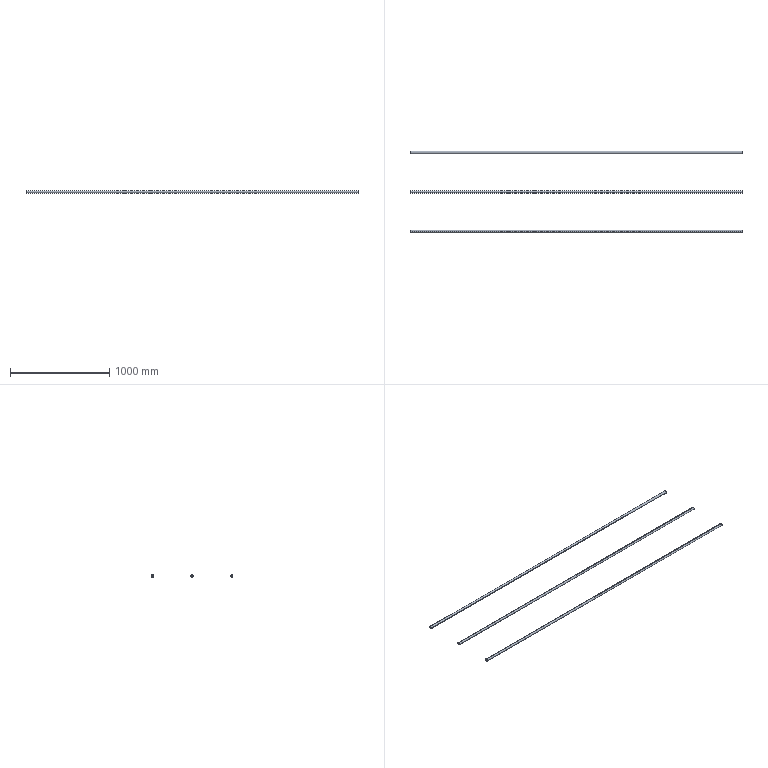Part | STEP file | 粉仓护栏栏杆7_Default<As Machined> | 3 solids | 18 faces | box 3350 x 825 x 25 mm | volume 1112948 mm3 | cylinder 12 | plane 6 | commonest cylinder face diameters 22 x6 25 x6
STEP:
#1=CARTESIAN_POINT('',(0.,0.,0.));
#2=DIRECTION('',(0.,0.,1.));
#3=DIRECTION('',(1.,0.,0.));
#4=AXIS2_PLACEMENT_3D('',#1,#2,#3);
#5=CARTESIAN_POINT('',(-3350.,0.,12.5));
#6=VERTEX_POINT('',#5);
#7=CARTESIAN_POINT('',(-3350.,0.,-12.5));
#8=VERTEX_POINT('',#7);
#9=CARTESIAN_POINT('',(-3350.,0.,0.));
#10=DIRECTION('',(-1.,0.,0.));
#11=DIRECTION('',(0.,-1.,0.));
#12=AXIS2_PLACEMENT_3D('',#9,#10,#11);
#13=CIRCLE('',#12,12.5);
#14=CARTESIAN_POINT('',(-3350.,0.,0.));
#15=DIRECTION('',(1.,0.,0.));
#16=DIRECTION('',(0.,0.,-1.));
#17=AXIS2_PLACEMENT_3D('',#14,#15,#16);
#18=CYLINDRICAL_SURFACE('',#17,12.5);
#19=CARTESIAN_POINT('',(4.712,0.));
#20=DIRECTION('',(-1.,0.));
#21=VECTOR('',#20,1.);
#22=LINE('',#19,#21);
#23=(GEOMETRIC_REPRESENTATION_CONTEXT(2)PARAMETRIC_REPRESENTATION_CONTEXT()REPRESENTATION_CONTEXT('',''));
#24=DEFINITIONAL_REPRESENTATION('',(#22),#23);
#25=PCURVE('',#18,#24);
#26=CARTESIAN_POINT('',(-3350.,0.,0.));
#27=DIRECTION('',(-1.,0.,0.));
#28=DIRECTION('',(0.,-1.,0.));
#29=AXIS2_PLACEMENT_3D('',#26,#27,#28);
#30=PLANE('',#29);
#31=CARTESIAN_POINT('',(0.,0.));
#32=DIRECTION('',(1.,0.));
#33=AXIS2_PLACEMENT_2D('',#31,#32);
#34=CIRCLE('',#33,12.5);
#35=(GEOMETRIC_REPRESENTATION_CONTEXT(2)PARAMETRIC_REPRESENTATION_CONTEXT()REPRESENTATION_CONTEXT('',''));
#36=DEFINITIONAL_REPRESENTATION('',(#34),#35);
#37=PCURVE('',#30,#36);
#38=SURFACE_CURVE('',#13,(#25,#37),.PCURVE_S1.);
#39=EDGE_CURVE('',#6,#8,#38,.T.);
#40=ORIENTED_EDGE('',*,*,#39,.F.);
#41=CARTESIAN_POINT('',(0.,0.,12.5));
#42=VERTEX_POINT('',#41);
#43=CARTESIAN_POINT('',(-3350.,0.,12.5));
#44=DIRECTION('',(1.,0.,0.));
#45=VECTOR('',#44,1.);
#46=LINE('',#43,#45);
#47=CARTESIAN_POINT('',(3.142,0.));
#48=DIRECTION('',(0.,1.));
#49=VECTOR('',#48,1.);
#50=LINE('',#47,#49);
#51=(GEOMETRIC_REPRESENTATION_CONTEXT(2)PARAMETRIC_REPRESENTATION_CONTEXT()REPRESENTATION_CONTEXT('',''));
#52=DEFINITIONAL_REPRESENTATION('',(#50),#51);
#53=PCURVE('',#18,#52);
#54=CARTESIAN_POINT('',(-3350.,0.,0.));
#55=DIRECTION('',(1.,0.,0.));
#56=DIRECTION('',(0.,0.,-1.));
#57=AXIS2_PLACEMENT_3D('',#54,#55,#56);
#58=CYLINDRICAL_SURFACE('',#57,12.5);
#59=CARTESIAN_POINT('',(3.142,0.));
#60=DIRECTION('',(0.,1.));
#61=VECTOR('',#60,1.);
#62=LINE('',#59,#61);
#63=(GEOMETRIC_REPRESENTATION_CONTEXT(2)PARAMETRIC_REPRESENTATION_CONTEXT()REPRESENTATION_CONTEXT('',''));
#64=DEFINITIONAL_REPRESENTATION('',(#62),#63);
#65=PCURVE('',#58,#64);
#66=SURFACE_CURVE('',#46,(#53,#65),.PCURVE_S1.);
#67=EDGE_CURVE('',#6,#42,#66,.T.);
#68=ORIENTED_EDGE('',*,*,#67,.T.);
#69=CARTESIAN_POINT('',(0.,0.,-12.5));
#70=VERTEX_POINT('',#69);
#71=CARTESIAN_POINT('',(0.,0.,0.));
#72=DIRECTION('',(-1.,0.,0.));
#73=DIRECTION('',(0.,-1.,0.));
#74=AXIS2_PLACEMENT_3D('',#71,#72,#73);
#75=CIRCLE('',#74,12.5);
#76=CARTESIAN_POINT('',(4.712,3350.));
#77=DIRECTION('',(-1.,0.));
#78=VECTOR('',#77,1.);
#79=LINE('',#76,#78);
#80=(GEOMETRIC_REPRESENTATION_CONTEXT(2)PARAMETRIC_REPRESENTATION_CONTEXT()REPRESENTATION_CONTEXT('',''));
#81=DEFINITIONAL_REPRESENTATION('',(#79),#80);
#82=PCURVE('',#18,#81);
#83=CARTESIAN_POINT('',(0.,0.,0.));
#84=DIRECTION('',(-1.,0.,0.));
#85=DIRECTION('',(0.,-1.,0.));
#86=AXIS2_PLACEMENT_3D('',#83,#84,#85);
#87=PLANE('',#86);
#88=CARTESIAN_POINT('',(0.,0.));
#89=DIRECTION('',(1.,0.));
#90=AXIS2_PLACEMENT_2D('',#88,#89);
#91=CIRCLE('',#90,12.5);
#92=(GEOMETRIC_REPRESENTATION_CONTEXT(2)PARAMETRIC_REPRESENTATION_CONTEXT()REPRESENTATION_CONTEXT('',''));
#93=DEFINITIONAL_REPRESENTATION('',(#91),#92);
#94=PCURVE('',#87,#93);
#95=SURFACE_CURVE('',#75,(#82,#94),.PCURVE_S1.);
#96=EDGE_CURVE('',#42,#70,#95,.T.);
#97=ORIENTED_EDGE('',*,*,#96,.T.);
#98=CARTESIAN_POINT('',(-3350.,0.,-12.5));
#99=DIRECTION('',(1.,0.,0.));
#100=VECTOR('',#99,1.);
#101=LINE('',#98,#100);
#102=CARTESIAN_POINT('',(0.,0.));
#103=DIRECTION('',(0.,1.));
#104=VECTOR('',#103,1.);
#105=LINE('',#102,#104);
#106=(GEOMETRIC_REPRESENTATION_CONTEXT(2)PARAMETRIC_REPRESENTATION_CONTEXT()REPRESENTATION_CONTEXT('',''));
#107=DEFINITIONAL_REPRESENTATION('',(#105),#106);
#108=PCURVE('',#18,#107);
#109=CARTESIAN_POINT('',(6.283,0.));
#110=DIRECTION('',(0.,1.));
#111=VECTOR('',#110,1.);
#112=LINE('',#109,#111);
#113=(GEOMETRIC_REPRESENTATION_CONTEXT(2)PARAMETRIC_REPRESENTATION_CONTEXT()REPRESENTATION_CONTEXT('',''));
#114=DEFINITIONAL_REPRESENTATION('',(#112),#113);
#115=PCURVE('',#58,#114);
#116=SURFACE_CURVE('',#101,(#108,#115),.PCURVE_S1.);
#117=EDGE_CURVE('',#8,#70,#116,.T.);
#118=ORIENTED_EDGE('',*,*,#117,.F.);
#119=EDGE_LOOP('',(#40,#68,#97,#118));
#120=FACE_BOUND('',#119,.T.);
#121=ADVANCED_FACE('',(#120),#18,.T.);
#122=CARTESIAN_POINT('',(-3350.,0.,-11.));
#123=VERTEX_POINT('',#122);
#124=CARTESIAN_POINT('',(0.,0.,-11.));
#125=VERTEX_POINT('',#124);
#126=CARTESIAN_POINT('',(-3350.,0.,-11.));
#127=DIRECTION('',(1.,0.,0.));
#128=VECTOR('',#127,1.);
#129=LINE('',#126,#128);
#130=CARTESIAN_POINT('',(-3350.,0.,0.));
#131=DIRECTION('',(1.,0.,0.));
#132=DIRECTION('',(0.,0.,-1.));
#133=AXIS2_PLACEMENT_3D('',#130,#131,#132);
#134=CYLINDRICAL_SURFACE('',#133,11.);
#135=CARTESIAN_POINT('',(6.283,0.));
#136=DIRECTION('',(0.,1.));
#137=VECTOR('',#136,1.);
#138=LINE('',#135,#137);
#139=(GEOMETRIC_REPRESENTATION_CONTEXT(2)PARAMETRIC_REPRESENTATION_CONTEXT()REPRESENTATION_CONTEXT('',''));
#140=DEFINITIONAL_REPRESENTATION('',(#138),#139);
#141=PCURVE('',#134,#140);
#142=CARTESIAN_POINT('',(-3350.,0.,0.));
#143=DIRECTION('',(1.,0.,0.));
#144=DIRECTION('',(0.,0.,-1.));
#145=AXIS2_PLACEMENT_3D('',#142,#143,#144);
#146=CYLINDRICAL_SURFACE('',#145,11.);
#147=CARTESIAN_POINT('',(0.,0.));
#148=DIRECTION('',(0.,1.));
#149=VECTOR('',#148,1.);
#150=LINE('',#147,#149);
#151=(GEOMETRIC_REPRESENTATION_CONTEXT(2)PARAMETRIC_REPRESENTATION_CONTEXT()REPRESENTATION_CONTEXT('',''));
#152=DEFINITIONAL_REPRESENTATION('',(#150),#151);
#153=PCURVE('',#146,#152);
#154=SURFACE_CURVE('',#129,(#141,#153),.PCURVE_S1.);
#155=EDGE_CURVE('',#123,#125,#154,.T.);
#156=ORIENTED_EDGE('',*,*,#155,.T.);
#157=CARTESIAN_POINT('',(0.,0.,11.));
#158=VERTEX_POINT('',#157);
#159=CARTESIAN_POINT('',(0.,0.,0.));
#160=DIRECTION('',(-1.,0.,0.));
#161=DIRECTION('',(0.,-1.,0.));
#162=AXIS2_PLACEMENT_3D('',#159,#160,#161);
#163=CIRCLE('',#162,11.);
#164=CARTESIAN_POINT('',(10.996,3350.));
#165=DIRECTION('',(-1.,0.));
#166=VECTOR('',#165,1.);
#167=LINE('',#164,#166);
#168=(GEOMETRIC_REPRESENTATION_CONTEXT(2)PARAMETRIC_REPRESENTATION_CONTEXT()REPRESENTATION_CONTEXT('',''));
#169=DEFINITIONAL_REPRESENTATION('',(#167),#168);
#170=PCURVE('',#134,#169);
#171=CARTESIAN_POINT('',(0.,0.));
#172=DIRECTION('',(1.,0.));
#173=AXIS2_PLACEMENT_2D('',#171,#172);
#174=CIRCLE('',#173,11.);
#175=(GEOMETRIC_REPRESENTATION_CONTEXT(2)PARAMETRIC_REPRESENTATION_CONTEXT()REPRESENTATION_CONTEXT('',''));
#176=DEFINITIONAL_REPRESENTATION('',(#174),#175);
#177=PCURVE('',#87,#176);
#178=SURFACE_CURVE('',#163,(#170,#177),.PCURVE_S1.);
#179=EDGE_CURVE('',#125,#158,#178,.T.);
#180=ORIENTED_EDGE('',*,*,#179,.T.);
#181=CARTESIAN_POINT('',(-3350.,0.,11.));
#182=VERTEX_POINT('',#181);
#183=CARTESIAN_POINT('',(-3350.,0.,11.));
#184=DIRECTION('',(1.,0.,0.));
#185=VECTOR('',#184,1.);
#186=LINE('',#183,#185);
#187=CARTESIAN_POINT('',(3.142,0.));
#188=DIRECTION('',(0.,1.));
#189=VECTOR('',#188,1.);
#190=LINE('',#187,#189);
#191=(GEOMETRIC_REPRESENTATION_CONTEXT(2)PARAMETRIC_REPRESENTATION_CONTEXT()REPRESENTATION_CONTEXT('',''));
#192=DEFINITIONAL_REPRESENTATION('',(#190),#191);
#193=PCURVE('',#134,#192);
#194=CARTESIAN_POINT('',(3.142,0.));
#195=DIRECTION('',(0.,1.));
#196=VECTOR('',#195,1.);
#197=LINE('',#194,#196);
#198=(GEOMETRIC_REPRESENTATION_CONTEXT(2)PARAMETRIC_REPRESENTATION_CONTEXT()REPRESENTATION_CONTEXT('',''));
#199=DEFINITIONAL_REPRESENTATION('',(#197),#198);
#200=PCURVE('',#146,#199);
#201=SURFACE_CURVE('',#186,(#193,#200),.PCURVE_S1.);
#202=EDGE_CURVE('',#182,#158,#201,.T.);
#203=ORIENTED_EDGE('',*,*,#202,.F.);
#204=CARTESIAN_POINT('',(-3350.,0.,0.));
#205=DIRECTION('',(-1.,0.,0.));
#206=DIRECTION('',(0.,-1.,0.));
#207=AXIS2_PLACEMENT_3D('',#204,#205,#206);
#208=CIRCLE('',#207,11.);
#209=CARTESIAN_POINT('',(10.996,0.));
#210=DIRECTION('',(-1.,0.));
#211=VECTOR('',#210,1.);
#212=LINE('',#209,#211);
#213=(GEOMETRIC_REPRESENTATION_CONTEXT(2)PARAMETRIC_REPRESENTATION_CONTEXT()REPRESENTATION_CONTEXT('',''));
#214=DEFINITIONAL_REPRESENTATION('',(#212),#213);
#215=PCURVE('',#134,#214);
#216=CARTESIAN_POINT('',(0.,0.));
#217=DIRECTION('',(1.,0.));
#218=AXIS2_PLACEMENT_2D('',#216,#217);
#219=CIRCLE('',#218,11.);
#220=(GEOMETRIC_REPRESENTATION_CONTEXT(2)PARAMETRIC_REPRESENTATION_CONTEXT()REPRESENTATION_CONTEXT('',''));
#221=DEFINITIONAL_REPRESENTATION('',(#219),#220);
#222=PCURVE('',#30,#221);
#223=SURFACE_CURVE('',#208,(#215,#222),.PCURVE_S1.);
#224=EDGE_CURVE('',#123,#182,#223,.T.);
#225=ORIENTED_EDGE('',*,*,#224,.F.);
#226=EDGE_LOOP('',(#156,#180,#203,#225));
#227=FACE_BOUND('',#226,.F.);
#228=ADVANCED_FACE('',(#227),#134,.F.);
#229=CARTESIAN_POINT('',(0.,0.,0.));
#230=DIRECTION('',(-1.,0.,0.));
#231=DIRECTION('',(0.,-1.,0.));
#232=AXIS2_PLACEMENT_3D('',#229,#230,#231);
#233=CIRCLE('',#232,11.);
#234=CARTESIAN_POINT('',(4.712,3350.));
#235=DIRECTION('',(-1.,0.));
#236=VECTOR('',#235,1.);
#237=LINE('',#234,#236);
#238=(GEOMETRIC_REPRESENTATION_CONTEXT(2)PARAMETRIC_REPRESENTATION_CONTEXT()REPRESENTATION_CONTEXT('',''));
#239=DEFINITIONAL_REPRESENTATION('',(#237),#238);
#240=PCURVE('',#146,#239);
#241=CARTESIAN_POINT('',(0.,0.));
#242=DIRECTION('',(1.,0.));
#243=AXIS2_PLACEMENT_2D('',#241,#242);
#244=CIRCLE('',#243,11.);
#245=(GEOMETRIC_REPRESENTATION_CONTEXT(2)PARAMETRIC_REPRESENTATION_CONTEXT()REPRESENTATION_CONTEXT('',''));
#246=DEFINITIONAL_REPRESENTATION('',(#244),#245);
#247=PCURVE('',#87,#246);
#248=SURFACE_CURVE('',#233,(#240,#247),.PCURVE_S1.);
#249=EDGE_CURVE('',#158,#125,#248,.T.);
#250=ORIENTED_EDGE('',*,*,#249,.T.);
#251=ORIENTED_EDGE('',*,*,#155,.F.);
#252=CARTESIAN_POINT('',(-3350.,0.,0.));
#253=DIRECTION('',(-1.,0.,0.));
#254=DIRECTION('',(0.,-1.,0.));
#255=AXIS2_PLACEMENT_3D('',#252,#253,#254);
#256=CIRCLE('',#255,11.);
#257=CARTESIAN_POINT('',(4.712,0.));
#258=DIRECTION('',(-1.,0.));
#259=VECTOR('',#258,1.);
#260=LINE('',#257,#259);
#261=(GEOMETRIC_REPRESENTATION_CONTEXT(2)PARAMETRIC_REPRESENTATION_CONTEXT()REPRESENTATION_CONTEXT('',''));
#262=DEFINITIONAL_REPRESENTATION('',(#260),#261);
#263=PCURVE('',#146,#262);
#264=CARTESIAN_POINT('',(0.,0.));
#265=DIRECTION('',(1.,0.));
#266=AXIS2_PLACEMENT_2D('',#264,#265);
#267=CIRCLE('',#266,11.);
#268=(GEOMETRIC_REPRESENTATION_CONTEXT(2)PARAMETRIC_REPRESENTATION_CONTEXT()REPRESENTATION_CONTEXT('',''));
#269=DEFINITIONAL_REPRESENTATION('',(#267),#268);
#270=PCURVE('',#30,#269);
#271=SURFACE_CURVE('',#256,(#263,#270),.PCURVE_S1.);
#272=EDGE_CURVE('',#182,#123,#271,.T.);
#273=ORIENTED_EDGE('',*,*,#272,.F.);
#274=ORIENTED_EDGE('',*,*,#202,.T.);
#275=EDGE_LOOP('',(#250,#251,#273,#274));
#276=FACE_BOUND('',#275,.F.);
#277=ADVANCED_FACE('',(#276),#146,.F.);
#278=ORIENTED_EDGE('',*,*,#67,.F.);
#279=CARTESIAN_POINT('',(-3350.,0.,0.));
#280=DIRECTION('',(-1.,0.,0.));
#281=DIRECTION('',(0.,-1.,0.));
#282=AXIS2_PLACEMENT_3D('',#279,#280,#281);
#283=CIRCLE('',#282,12.5);
#284=CARTESIAN_POINT('',(10.996,0.));
#285=DIRECTION('',(-1.,0.));
#286=VECTOR('',#285,1.);
#287=LINE('',#284,#286);
#288=(GEOMETRIC_REPRESENTATION_CONTEXT(2)PARAMETRIC_REPRESENTATION_CONTEXT()REPRESENTATION_CONTEXT('',''));
#289=DEFINITIONAL_REPRESENTATION('',(#287),#288);
#290=PCURVE('',#58,#289);
#291=CARTESIAN_POINT('',(0.,0.));
#292=DIRECTION('',(1.,0.));
#293=AXIS2_PLACEMENT_2D('',#291,#292);
#294=CIRCLE('',#293,12.5);
#295=(GEOMETRIC_REPRESENTATION_CONTEXT(2)PARAMETRIC_REPRESENTATION_CONTEXT()REPRESENTATION_CONTEXT('',''));
#296=DEFINITIONAL_REPRESENTATION('',(#294),#295);
#297=PCURVE('',#30,#296);
#298=SURFACE_CURVE('',#283,(#290,#297),.PCURVE_S1.);
#299=EDGE_CURVE('',#8,#6,#298,.T.);
#300=ORIENTED_EDGE('',*,*,#299,.F.);
#301=ORIENTED_EDGE('',*,*,#117,.T.);
#302=CARTESIAN_POINT('',(0.,0.,0.));
#303=DIRECTION('',(-1.,0.,0.));
#304=DIRECTION('',(0.,-1.,0.));
#305=AXIS2_PLACEMENT_3D('',#302,#303,#304);
#306=CIRCLE('',#305,12.5);
#307=CARTESIAN_POINT('',(10.996,3350.));
#308=DIRECTION('',(-1.,0.));
#309=VECTOR('',#308,1.);
#310=LINE('',#307,#309);
#311=(GEOMETRIC_REPRESENTATION_CONTEXT(2)PARAMETRIC_REPRESENTATION_CONTEXT()REPRESENTATION_CONTEXT('',''));
#312=DEFINITIONAL_REPRESENTATION('',(#310),#311);
#313=PCURVE('',#58,#312);
#314=CARTESIAN_POINT('',(0.,0.));
#315=DIRECTION('',(1.,0.));
#316=AXIS2_PLACEMENT_2D('',#314,#315);
#317=CIRCLE('',#316,12.5);
#318=(GEOMETRIC_REPRESENTATION_CONTEXT(2)PARAMETRIC_REPRESENTATION_CONTEXT()REPRESENTATION_CONTEXT('',''));
#319=DEFINITIONAL_REPRESENTATION('',(#317),#318);
#320=PCURVE('',#87,#319);
#321=SURFACE_CURVE('',#306,(#313,#320),.PCURVE_S1.);
#322=EDGE_CURVE('',#70,#42,#321,.T.);
#323=ORIENTED_EDGE('',*,*,#322,.T.);
#324=EDGE_LOOP('',(#278,#300,#301,#323));
#325=FACE_BOUND('',#324,.T.);
#326=ADVANCED_FACE('',(#325),#58,.T.);
#327=ORIENTED_EDGE('',*,*,#224,.F.);
#328=ORIENTED_EDGE('',*,*,#272,.F.);
#329=EDGE_LOOP('',(#327,#328));
#330=FACE_BOUND('',#329,.T.);
#331=ORIENTED_EDGE('',*,*,#299,.T.);
#332=ORIENTED_EDGE('',*,*,#39,.T.);
#333=EDGE_LOOP('',(#331,#332));
#334=FACE_BOUND('',#333,.T.);
#335=ADVANCED_FACE('',(#330,#334),#30,.T.);
#336=ORIENTED_EDGE('',*,*,#179,.T.);
#337=ORIENTED_EDGE('',*,*,#249,.T.);
#338=EDGE_LOOP('',(#336,#337));
#339=FACE_BOUND('',#338,.T.);
#340=ORIENTED_EDGE('',*,*,#322,.F.);
#341=ORIENTED_EDGE('',*,*,#96,.F.);
#342=EDGE_LOOP('',(#340,#341));
#343=FACE_BOUND('',#342,.T.);
#344=ADVANCED_FACE('',(#339,#343),#87,.F.);
#345=CLOSED_SHELL('',(#121,#228,#277,#326,#335,#344));
#346=MANIFOLD_SOLID_BREP('',#345);
#347=CARTESIAN_POINT('',(-3350.,787.5,0.));
#348=VERTEX_POINT('',#347);
#349=CARTESIAN_POINT('',(-3350.,812.5,0.));
#350=VERTEX_POINT('',#349);
#351=CARTESIAN_POINT('',(-3350.,800.,0.));
#352=DIRECTION('',(-1.,0.,0.));
#353=DIRECTION('',(0.,-1.,0.));
#354=AXIS2_PLACEMENT_3D('',#351,#352,#353);
#355=CIRCLE('',#354,12.5);
#356=CARTESIAN_POINT('',(-3350.,800.,0.));
#357=DIRECTION('',(1.,0.,0.));
#358=DIRECTION('',(0.,1.,0.));
#359=AXIS2_PLACEMENT_3D('',#356,#357,#358);
#360=CYLINDRICAL_SURFACE('',#359,12.5);
#361=CARTESIAN_POINT('',(3.142,0.));
#362=DIRECTION('',(-1.,0.));
#363=VECTOR('',#362,1.);
#364=LINE('',#361,#363);
#365=(GEOMETRIC_REPRESENTATION_CONTEXT(2)PARAMETRIC_REPRESENTATION_CONTEXT()REPRESENTATION_CONTEXT('',''));
#366=DEFINITIONAL_REPRESENTATION('',(#364),#365);
#367=PCURVE('',#360,#366);
#368=CARTESIAN_POINT('',(-3350.,800.,0.));
#369=DIRECTION('',(-1.,0.,0.));
#370=DIRECTION('',(0.,-1.,0.));
#371=AXIS2_PLACEMENT_3D('',#368,#369,#370);
#372=PLANE('',#371);
#373=CARTESIAN_POINT('',(0.,0.));
#374=DIRECTION('',(1.,0.));
#375=AXIS2_PLACEMENT_2D('',#373,#374);
#376=CIRCLE('',#375,12.5);
#377=(GEOMETRIC_REPRESENTATION_CONTEXT(2)PARAMETRIC_REPRESENTATION_CONTEXT()REPRESENTATION_CONTEXT('',''));
#378=DEFINITIONAL_REPRESENTATION('',(#376),#377);
#379=PCURVE('',#372,#378);
#380=SURFACE_CURVE('',#355,(#367,#379),.PCURVE_S1.);
#381=EDGE_CURVE('',#348,#350,#380,.T.);
#382=ORIENTED_EDGE('',*,*,#381,.F.);
#383=CARTESIAN_POINT('',(0.,787.5,0.));
#384=VERTEX_POINT('',#383);
#385=CARTESIAN_POINT('',(-3350.,787.5,0.));
#386=DIRECTION('',(1.,0.,0.));
#387=VECTOR('',#386,1.);
#388=LINE('',#385,#387);
#389=CARTESIAN_POINT('',(3.142,0.));
#390=DIRECTION('',(0.,1.));
#391=VECTOR('',#390,1.);
#392=LINE('',#389,#391);
#393=(GEOMETRIC_REPRESENTATION_CONTEXT(2)PARAMETRIC_REPRESENTATION_CONTEXT()REPRESENTATION_CONTEXT('',''));
#394=DEFINITIONAL_REPRESENTATION('',(#392),#393);
#395=PCURVE('',#360,#394);
#396=CARTESIAN_POINT('',(-3350.,800.,0.));
#397=DIRECTION('',(1.,0.,0.));
#398=DIRECTION('',(0.,1.,0.));
#399=AXIS2_PLACEMENT_3D('',#396,#397,#398);
#400=CYLINDRICAL_SURFACE('',#399,12.5);
#401=CARTESIAN_POINT('',(3.142,0.));
#402=DIRECTION('',(0.,1.));
#403=VECTOR('',#402,1.);
#404=LINE('',#401,#403);
#405=(GEOMETRIC_REPRESENTATION_CONTEXT(2)PARAMETRIC_REPRESENTATION_CONTEXT()REPRESENTATION_CONTEXT('',''));
#406=DEFINITIONAL_REPRESENTATION('',(#404),#405);
#407=PCURVE('',#400,#406);
#408=SURFACE_CURVE('',#388,(#395,#407),.PCURVE_S1.);
#409=EDGE_CURVE('',#348,#384,#408,.T.);
#410=ORIENTED_EDGE('',*,*,#409,.T.);
#411=CARTESIAN_POINT('',(0.,812.5,0.));
#412=VERTEX_POINT('',#411);
#413=CARTESIAN_POINT('',(0.,800.,0.));
#414=DIRECTION('',(-1.,0.,0.));
#415=DIRECTION('',(0.,-1.,0.));
#416=AXIS2_PLACEMENT_3D('',#413,#414,#415);
#417=CIRCLE('',#416,12.5);
#418=CARTESIAN_POINT('',(3.142,3350.));
#419=DIRECTION('',(-1.,0.));
#420=VECTOR('',#419,1.);
#421=LINE('',#418,#420);
#422=(GEOMETRIC_REPRESENTATION_CONTEXT(2)PARAMETRIC_REPRESENTATION_CONTEXT()REPRESENTATION_CONTEXT('',''));
#423=DEFINITIONAL_REPRESENTATION('',(#421),#422);
#424=PCURVE('',#360,#423);
#425=CARTESIAN_POINT('',(0.,800.,0.));
#426=DIRECTION('',(-1.,0.,0.));
#427=DIRECTION('',(0.,-1.,0.));
#428=AXIS2_PLACEMENT_3D('',#425,#426,#427);
#429=PLANE('',#428);
#430=CARTESIAN_POINT('',(0.,0.));
#431=DIRECTION('',(1.,0.));
#432=AXIS2_PLACEMENT_2D('',#430,#431);
#433=CIRCLE('',#432,12.5);
#434=(GEOMETRIC_REPRESENTATION_CONTEXT(2)PARAMETRIC_REPRESENTATION_CONTEXT()REPRESENTATION_CONTEXT('',''));
#435=DEFINITIONAL_REPRESENTATION('',(#433),#434);
#436=PCURVE('',#429,#435);
#437=SURFACE_CURVE('',#417,(#424,#436),.PCURVE_S1.);
#438=EDGE_CURVE('',#384,#412,#437,.T.);
#439=ORIENTED_EDGE('',*,*,#438,.T.);
#440=CARTESIAN_POINT('',(-3350.,812.5,0.));
#441=DIRECTION('',(1.,0.,0.));
#442=VECTOR('',#441,1.);
#443=LINE('',#440,#442);
#444=CARTESIAN_POINT('',(0.,0.));
#445=DIRECTION('',(0.,1.));
#446=VECTOR('',#445,1.);
#447=LINE('',#444,#446);
#448=(GEOMETRIC_REPRESENTATION_CONTEXT(2)PARAMETRIC_REPRESENTATION_CONTEXT()REPRESENTATION_CONTEXT('',''));
#449=DEFINITIONAL_REPRESENTATION('',(#447),#448);
#450=PCURVE('',#360,#449);
#451=CARTESIAN_POINT('',(6.283,0.));
#452=DIRECTION('',(0.,1.));
#453=VECTOR('',#452,1.);
#454=LINE('',#451,#453);
#455=(GEOMETRIC_REPRESENTATION_CONTEXT(2)PARAMETRIC_REPRESENTATION_CONTEXT()REPRESENTATION_CONTEXT('',''));
#456=DEFINITIONAL_REPRESENTATION('',(#454),#455);
#457=PCURVE('',#400,#456);
#458=SURFACE_CURVE('',#443,(#450,#457),.PCURVE_S1.);
#459=EDGE_CURVE('',#350,#412,#458,.T.);
#460=ORIENTED_EDGE('',*,*,#459,.F.);
#461=EDGE_LOOP('',(#382,#410,#439,#460));
#462=FACE_BOUND('',#461,.T.);
#463=ADVANCED_FACE('',(#462),#360,.T.);
#464=CARTESIAN_POINT('',(-3350.,811.,0.));
#465=VERTEX_POINT('',#464);
#466=CARTESIAN_POINT('',(0.,811.,0.));
#467=VERTEX_POINT('',#466);
#468=CARTESIAN_POINT('',(-3350.,811.,0.));
#469=DIRECTION('',(1.,0.,0.));
#470=VECTOR('',#469,1.);
#471=LINE('',#468,#470);
#472=CARTESIAN_POINT('',(-3350.,800.,0.));
#473=DIRECTION('',(1.,0.,0.));
#474=DIRECTION('',(0.,1.,0.));
#475=AXIS2_PLACEMENT_3D('',#472,#473,#474);
#476=CYLINDRICAL_SURFACE('',#475,11.);
#477=CARTESIAN_POINT('',(6.283,0.));
#478=DIRECTION('',(0.,1.));
#479=VECTOR('',#478,1.);
#480=LINE('',#477,#479);
#481=(GEOMETRIC_REPRESENTATION_CONTEXT(2)PARAMETRIC_REPRESENTATION_CONTEXT()REPRESENTATION_CONTEXT('',''));
#482=DEFINITIONAL_REPRESENTATION('',(#480),#481);
#483=PCURVE('',#476,#482);
#484=CARTESIAN_POINT('',(-3350.,800.,0.));
#485=DIRECTION('',(1.,0.,0.));
#486=DIRECTION('',(0.,1.,0.));
#487=AXIS2_PLACEMENT_3D('',#484,#485,#486);
#488=CYLINDRICAL_SURFACE('',#487,11.);
#489=CARTESIAN_POINT('',(0.,0.));
#490=DIRECTION('',(0.,1.));
#491=VECTOR('',#490,1.);
#492=LINE('',#489,#491);
#493=(GEOMETRIC_REPRESENTATION_CONTEXT(2)PARAMETRIC_REPRESENTATION_CONTEXT()REPRESENTATION_CONTEXT('',''));
#494=DEFINITIONAL_REPRESENTATION('',(#492),#493);
#495=PCURVE('',#488,#494);
#496=SURFACE_CURVE('',#471,(#483,#495),.PCURVE_S1.);
#497=EDGE_CURVE('',#465,#467,#496,.T.);
#498=ORIENTED_EDGE('',*,*,#497,.T.);
#499=CARTESIAN_POINT('',(0.,789.,0.));
#500=VERTEX_POINT('',#499);
#501=CARTESIAN_POINT('',(0.,800.,0.));
#502=DIRECTION('',(-1.,0.,0.));
#503=DIRECTION('',(0.,-1.,0.));
#504=AXIS2_PLACEMENT_3D('',#501,#502,#503);
#505=CIRCLE('',#504,11.);
#506=CARTESIAN_POINT('',(9.425,3350.));
#507=DIRECTION('',(-1.,0.));
#508=VECTOR('',#507,1.);
#509=LINE('',#506,#508);
#510=(GEOMETRIC_REPRESENTATION_CONTEXT(2)PARAMETRIC_REPRESENTATION_CONTEXT()REPRESENTATION_CONTEXT('',''));
#511=DEFINITIONAL_REPRESENTATION('',(#509),#510);
#512=PCURVE('',#476,#511);
#513=CARTESIAN_POINT('',(0.,0.));
#514=DIRECTION('',(1.,0.));
#515=AXIS2_PLACEMENT_2D('',#513,#514);
#516=CIRCLE('',#515,11.);
#517=(GEOMETRIC_REPRESENTATION_CONTEXT(2)PARAMETRIC_REPRESENTATION_CONTEXT()REPRESENTATION_CONTEXT('',''));
#518=DEFINITIONAL_REPRESENTATION('',(#516),#517);
#519=PCURVE('',#429,#518);
#520=SURFACE_CURVE('',#505,(#512,#519),.PCURVE_S1.);
#521=EDGE_CURVE('',#467,#500,#520,.T.);
#522=ORIENTED_EDGE('',*,*,#521,.T.);
#523=CARTESIAN_POINT('',(-3350.,789.,0.));
#524=VERTEX_POINT('',#523);
#525=CARTESIAN_POINT('',(-3350.,789.,0.));
#526=DIRECTION('',(1.,0.,0.));
#527=VECTOR('',#526,1.);
#528=LINE('',#525,#527);
#529=CARTESIAN_POINT('',(3.142,0.));
#530=DIRECTION('',(0.,1.));
#531=VECTOR('',#530,1.);
#532=LINE('',#529,#531);
#533=(GEOMETRIC_REPRESENTATION_CONTEXT(2)PARAMETRIC_REPRESENTATION_CONTEXT()REPRESENTATION_CONTEXT('',''));
#534=DEFINITIONAL_REPRESENTATION('',(#532),#533);
#535=PCURVE('',#476,#534);
#536=CARTESIAN_POINT('',(3.142,0.));
#537=DIRECTION('',(0.,1.));
#538=VECTOR('',#537,1.);
#539=LINE('',#536,#538);
#540=(GEOMETRIC_REPRESENTATION_CONTEXT(2)PARAMETRIC_REPRESENTATION_CONTEXT()REPRESENTATION_CONTEXT('',''));
#541=DEFINITIONAL_REPRESENTATION('',(#539),#540);
#542=PCURVE('',#488,#541);
#543=SURFACE_CURVE('',#528,(#535,#542),.PCURVE_S1.);
#544=EDGE_CURVE('',#524,#500,#543,.T.);
#545=ORIENTED_EDGE('',*,*,#544,.F.);
#546=CARTESIAN_POINT('',(-3350.,800.,0.));
#547=DIRECTION('',(-1.,0.,0.));
#548=DIRECTION('',(0.,-1.,0.));
#549=AXIS2_PLACEMENT_3D('',#546,#547,#548);
#550=CIRCLE('',#549,11.);
#551=CARTESIAN_POINT('',(9.425,0.));
#552=DIRECTION('',(-1.,0.));
#553=VECTOR('',#552,1.);
#554=LINE('',#551,#553);
#555=(GEOMETRIC_REPRESENTATION_CONTEXT(2)PARAMETRIC_REPRESENTATION_CONTEXT()REPRESENTATION_CONTEXT('',''));
#556=DEFINITIONAL_REPRESENTATION('',(#554),#555);
#557=PCURVE('',#476,#556);
#558=CARTESIAN_POINT('',(0.,0.));
#559=DIRECTION('',(1.,0.));
#560=AXIS2_PLACEMENT_2D('',#558,#559);
#561=CIRCLE('',#560,11.);
#562=(GEOMETRIC_REPRESENTATION_CONTEXT(2)PARAMETRIC_REPRESENTATION_CONTEXT()REPRESENTATION_CONTEXT('',''));
#563=DEFINITIONAL_REPRESENTATION('',(#561),#562);
#564=PCURVE('',#372,#563);
#565=SURFACE_CURVE('',#550,(#557,#564),.PCURVE_S1.);
#566=EDGE_CURVE('',#465,#524,#565,.T.);
#567=ORIENTED_EDGE('',*,*,#566,.F.);
#568=EDGE_LOOP('',(#498,#522,#545,#567));
#569=FACE_BOUND('',#568,.F.);
#570=ADVANCED_FACE('',(#569),#476,.F.);
#571=CARTESIAN_POINT('',(0.,800.,0.));
#572=DIRECTION('',(-1.,0.,0.));
#573=DIRECTION('',(0.,-1.,0.));
#574=AXIS2_PLACEMENT_3D('',#571,#572,#573);
#575=CIRCLE('',#574,11.);
#576=CARTESIAN_POINT('',(3.142,3350.));
#577=DIRECTION('',(-1.,0.));
#578=VECTOR('',#577,1.);
#579=LINE('',#576,#578);
#580=(GEOMETRIC_REPRESENTATION_CONTEXT(2)PARAMETRIC_REPRESENTATION_CONTEXT()REPRESENTATION_CONTEXT('',''));
#581=DEFINITIONAL_REPRESENTATION('',(#579),#580);
#582=PCURVE('',#488,#581);
#583=CARTESIAN_POINT('',(0.,0.));
#584=DIRECTION('',(1.,0.));
#585=AXIS2_PLACEMENT_2D('',#583,#584);
#586=CIRCLE('',#585,11.);
#587=(GEOMETRIC_REPRESENTATION_CONTEXT(2)PARAMETRIC_REPRESENTATION_CONTEXT()REPRESENTATION_CONTEXT('',''));
#588=DEFINITIONAL_REPRESENTATION('',(#586),#587);
#589=PCURVE('',#429,#588);
#590=SURFACE_CURVE('',#575,(#582,#589),.PCURVE_S1.);
#591=EDGE_CURVE('',#500,#467,#590,.T.);
#592=ORIENTED_EDGE('',*,*,#591,.T.);
#593=ORIENTED_EDGE('',*,*,#497,.F.);
#594=CARTESIAN_POINT('',(-3350.,800.,0.));
#595=DIRECTION('',(-1.,0.,0.));
#596=DIRECTION('',(0.,-1.,0.));
#597=AXIS2_PLACEMENT_3D('',#594,#595,#596);
#598=CIRCLE('',#597,11.);
#599=CARTESIAN_POINT('',(3.142,0.));
#600=DIRECTION('',(-1.,0.));
#601=VECTOR('',#600,1.);
#602=LINE('',#599,#601);
#603=(GEOMETRIC_REPRESENTATION_CONTEXT(2)PARAMETRIC_REPRESENTATION_CONTEXT()REPRESENTATION_CONTEXT('',''));
#604=DEFINITIONAL_REPRESENTATION('',(#602),#603);
#605=PCURVE('',#488,#604);
#606=CARTESIAN_POINT('',(0.,0.));
#607=DIRECTION('',(1.,0.));
#608=AXIS2_PLACEMENT_2D('',#606,#607);
#609=CIRCLE('',#608,11.);
#610=(GEOMETRIC_REPRESENTATION_CONTEXT(2)PARAMETRIC_REPRESENTATION_CONTEXT()REPRESENTATION_CONTEXT('',''));
#611=DEFINITIONAL_REPRESENTATION('',(#609),#610);
#612=PCURVE('',#372,#611);
#613=SURFACE_CURVE('',#598,(#605,#612),.PCURVE_S1.);
#614=EDGE_CURVE('',#524,#465,#613,.T.);
#615=ORIENTED_EDGE('',*,*,#614,.F.);
#616=ORIENTED_EDGE('',*,*,#544,.T.);
#617=EDGE_LOOP('',(#592,#593,#615,#616));
#618=FACE_BOUND('',#617,.F.);
#619=ADVANCED_FACE('',(#618),#488,.F.);
#620=ORIENTED_EDGE('',*,*,#409,.F.);
#621=CARTESIAN_POINT('',(-3350.,800.,0.));
#622=DIRECTION('',(-1.,0.,0.));
#623=DIRECTION('',(0.,-1.,0.));
#624=AXIS2_PLACEMENT_3D('',#621,#622,#623);
#625=CIRCLE('',#624,12.5);
#626=CARTESIAN_POINT('',(9.425,0.));
#627=DIRECTION('',(-1.,0.));
#628=VECTOR('',#627,1.);
#629=LINE('',#626,#628);
#630=(GEOMETRIC_REPRESENTATION_CONTEXT(2)PARAMETRIC_REPRESENTATION_CONTEXT()REPRESENTATION_CONTEXT('',''));
#631=DEFINITIONAL_REPRESENTATION('',(#629),#630);
#632=PCURVE('',#400,#631);
#633=CARTESIAN_POINT('',(0.,0.));
#634=DIRECTION('',(1.,0.));
#635=AXIS2_PLACEMENT_2D('',#633,#634);
#636=CIRCLE('',#635,12.5);
#637=(GEOMETRIC_REPRESENTATION_CONTEXT(2)PARAMETRIC_REPRESENTATION_CONTEXT()REPRESENTATION_CONTEXT('',''));
#638=DEFINITIONAL_REPRESENTATION('',(#636),#637);
#639=PCURVE('',#372,#638);
#640=SURFACE_CURVE('',#625,(#632,#639),.PCURVE_S1.);
#641=EDGE_CURVE('',#350,#348,#640,.T.);
#642=ORIENTED_EDGE('',*,*,#641,.F.);
#643=ORIENTED_EDGE('',*,*,#459,.T.);
#644=CARTESIAN_POINT('',(0.,800.,0.));
#645=DIRECTION('',(-1.,0.,0.));
#646=DIRECTION('',(0.,-1.,0.));
#647=AXIS2_PLACEMENT_3D('',#644,#645,#646);
#648=CIRCLE('',#647,12.5);
#649=CARTESIAN_POINT('',(9.425,3350.));
#650=DIRECTION('',(-1.,0.));
#651=VECTOR('',#650,1.);
#652=LINE('',#649,#651);
#653=(GEOMETRIC_REPRESENTATION_CONTEXT(2)PARAMETRIC_REPRESENTATION_CONTEXT()REPRESENTATION_CONTEXT('',''));
#654=DEFINITIONAL_REPRESENTATION('',(#652),#653);
#655=PCURVE('',#400,#654);
#656=CARTESIAN_POINT('',(0.,0.));
#657=DIRECTION('',(1.,0.));
#658=AXIS2_PLACEMENT_2D('',#656,#657);
#659=CIRCLE('',#658,12.5);
#660=(GEOMETRIC_REPRESENTATION_CONTEXT(2)PARAMETRIC_REPRESENTATION_CONTEXT()REPRESENTATION_CONTEXT('',''));
#661=DEFINITIONAL_REPRESENTATION('',(#659),#660);
#662=PCURVE('',#429,#661);
#663=SURFACE_CURVE('',#648,(#655,#662),.PCURVE_S1.);
#664=EDGE_CURVE('',#412,#384,#663,.T.);
#665=ORIENTED_EDGE('',*,*,#664,.T.);
#666=EDGE_LOOP('',(#620,#642,#643,#665));
#667=FACE_BOUND('',#666,.T.);
#668=ADVANCED_FACE('',(#667),#400,.T.);
#669=ORIENTED_EDGE('',*,*,#566,.F.);
#670=ORIENTED_EDGE('',*,*,#614,.F.);
#671=EDGE_LOOP('',(#669,#670));
#672=FACE_BOUND('',#671,.T.);
#673=ORIENTED_EDGE('',*,*,#641,.T.);
#674=ORIENTED_EDGE('',*,*,#381,.T.);
#675=EDGE_LOOP('',(#673,#674));
#676=FACE_BOUND('',#675,.T.);
#677=ADVANCED_FACE('',(#672,#676),#372,.T.);
#678=ORIENTED_EDGE('',*,*,#521,.T.);
#679=ORIENTED_EDGE('',*,*,#591,.T.);
#680=EDGE_LOOP('',(#678,#679));
#681=FACE_BOUND('',#680,.T.);
#682=ORIENTED_EDGE('',*,*,#664,.F.);
#683=ORIENTED_EDGE('',*,*,#438,.F.);
#684=EDGE_LOOP('',(#682,#683));
#685=FACE_BOUND('',#684,.T.);
#686=ADVANCED_FACE('',(#681,#685),#429,.F.);
#687=CLOSED_SHELL('',(#463,#570,#619,#668,#677,#686));
#688=MANIFOLD_SOLID_BREP('',#687);
#689=CARTESIAN_POINT('',(0.,400.,-12.5));
#690=VERTEX_POINT('',#689);
#691=CARTESIAN_POINT('',(0.,400.,12.5));
#692=VERTEX_POINT('',#691);
#693=CARTESIAN_POINT('',(0.,400.,0.));
#694=DIRECTION('',(1.,0.,0.));
#695=DIRECTION('',(0.,1.,0.));
#696=AXIS2_PLACEMENT_3D('',#693,#694,#695);
#697=CIRCLE('',#696,12.5);
#698=CARTESIAN_POINT('',(0.,400.,0.));
#699=DIRECTION('',(-1.,0.,0.));
#700=DIRECTION('',(0.,0.,1.));
#701=AXIS2_PLACEMENT_3D('',#698,#699,#700);
#702=CYLINDRICAL_SURFACE('',#701,12.5);
#703=CARTESIAN_POINT('',(7.854,0.));
#704=DIRECTION('',(-1.,0.));
#705=VECTOR('',#704,1.);
#706=LINE('',#703,#705);
#707=(GEOMETRIC_REPRESENTATION_CONTEXT(2)PARAMETRIC_REPRESENTATION_CONTEXT()REPRESENTATION_CONTEXT('',''));
#708=DEFINITIONAL_REPRESENTATION('',(#706),#707);
#709=PCURVE('',#702,#708);
#710=CARTESIAN_POINT('',(0.,400.,0.));
#711=DIRECTION('',(1.,0.,0.));
#712=DIRECTION('',(0.,1.,0.));
#713=AXIS2_PLACEMENT_3D('',#710,#711,#712);
#714=PLANE('',#713);
#715=CARTESIAN_POINT('',(0.,0.));
#716=DIRECTION('',(1.,0.));
#717=AXIS2_PLACEMENT_2D('',#715,#716);
#718=CIRCLE('',#717,12.5);
#719=(GEOMETRIC_REPRESENTATION_CONTEXT(2)PARAMETRIC_REPRESENTATION_CONTEXT()REPRESENTATION_CONTEXT('',''));
#720=DEFINITIONAL_REPRESENTATION('',(#718),#719);
#721=PCURVE('',#714,#720);
#722=SURFACE_CURVE('',#697,(#709,#721),.PCURVE_S1.);
#723=EDGE_CURVE('',#690,#692,#722,.T.);
#724=ORIENTED_EDGE('',*,*,#723,.F.);
#725=CARTESIAN_POINT('',(-3350.,400.,-12.5));
#726=VERTEX_POINT('',#725);
#727=CARTESIAN_POINT('',(0.,400.,-12.5));
#728=DIRECTION('',(-1.,0.,0.));
#729=VECTOR('',#728,1.);
#730=LINE('',#727,#729);
#731=CARTESIAN_POINT('',(3.142,0.));
#732=DIRECTION('',(0.,1.));
#733=VECTOR('',#732,1.);
#734=LINE('',#731,#733);
#735=(GEOMETRIC_REPRESENTATION_CONTEXT(2)PARAMETRIC_REPRESENTATION_CONTEXT()REPRESENTATION_CONTEXT('',''));
#736=DEFINITIONAL_REPRESENTATION('',(#734),#735);
#737=PCURVE('',#702,#736);
#738=CARTESIAN_POINT('',(0.,400.,0.));
#739=DIRECTION('',(-1.,0.,0.));
#740=DIRECTION('',(0.,0.,1.));
#741=AXIS2_PLACEMENT_3D('',#738,#739,#740);
#742=CYLINDRICAL_SURFACE('',#741,12.5);
#743=CARTESIAN_POINT('',(3.142,0.));
#744=DIRECTION('',(0.,1.));
#745=VECTOR('',#744,1.);
#746=LINE('',#743,#745);
#747=(GEOMETRIC_REPRESENTATION_CONTEXT(2)PARAMETRIC_REPRESENTATION_CONTEXT()REPRESENTATION_CONTEXT('',''));
#748=DEFINITIONAL_REPRESENTATION('',(#746),#747);
#749=PCURVE('',#742,#748);
#750=SURFACE_CURVE('',#730,(#737,#749),.PCURVE_S1.);
#751=EDGE_CURVE('',#690,#726,#750,.T.);
#752=ORIENTED_EDGE('',*,*,#751,.T.);
#753=CARTESIAN_POINT('',(-3350.,400.,12.5));
#754=VERTEX_POINT('',#753);
#755=CARTESIAN_POINT('',(-3350.,400.,0.));
#756=DIRECTION('',(1.,0.,0.));
#757=DIRECTION('',(0.,1.,0.));
#758=AXIS2_PLACEMENT_3D('',#755,#756,#757);
#759=CIRCLE('',#758,12.5);
#760=CARTESIAN_POINT('',(7.854,3350.));
#761=DIRECTION('',(-1.,0.));
#762=VECTOR('',#761,1.);
#763=LINE('',#760,#762);
#764=(GEOMETRIC_REPRESENTATION_CONTEXT(2)PARAMETRIC_REPRESENTATION_CONTEXT()REPRESENTATION_CONTEXT('',''));
#765=DEFINITIONAL_REPRESENTATION('',(#763),#764);
#766=PCURVE('',#702,#765);
#767=CARTESIAN_POINT('',(-3350.,400.,0.));
#768=DIRECTION('',(1.,0.,0.));
#769=DIRECTION('',(0.,1.,0.));
#770=AXIS2_PLACEMENT_3D('',#767,#768,#769);
#771=PLANE('',#770);
#772=CARTESIAN_POINT('',(0.,0.));
#773=DIRECTION('',(1.,0.));
#774=AXIS2_PLACEMENT_2D('',#772,#773);
#775=CIRCLE('',#774,12.5);
#776=(GEOMETRIC_REPRESENTATION_CONTEXT(2)PARAMETRIC_REPRESENTATION_CONTEXT()REPRESENTATION_CONTEXT('',''));
#777=DEFINITIONAL_REPRESENTATION('',(#775),#776);
#778=PCURVE('',#771,#777);
#779=SURFACE_CURVE('',#759,(#766,#778),.PCURVE_S1.);
#780=EDGE_CURVE('',#726,#754,#779,.T.);
#781=ORIENTED_EDGE('',*,*,#780,.T.);
#782=CARTESIAN_POINT('',(0.,400.,12.5));
#783=DIRECTION('',(-1.,0.,0.));
#784=VECTOR('',#783,1.);
#785=LINE('',#782,#784);
#786=CARTESIAN_POINT('',(0.,0.));
#787=DIRECTION('',(0.,1.));
#788=VECTOR('',#787,1.);
#789=LINE('',#786,#788);
#790=(GEOMETRIC_REPRESENTATION_CONTEXT(2)PARAMETRIC_REPRESENTATION_CONTEXT()REPRESENTATION_CONTEXT('',''));
#791=DEFINITIONAL_REPRESENTATION('',(#789),#790);
#792=PCURVE('',#702,#791);
#793=CARTESIAN_POINT('',(6.283,0.));
#794=DIRECTION('',(0.,1.));
#795=VECTOR('',#794,1.);
#796=LINE('',#793,#795);
#797=(GEOMETRIC_REPRESENTATION_CONTEXT(2)PARAMETRIC_REPRESENTATION_CONTEXT()REPRESENTATION_CONTEXT('',''));
#798=DEFINITIONAL_REPRESENTATION('',(#796),#797);
#799=PCURVE('',#742,#798);
#800=SURFACE_CURVE('',#785,(#792,#799),.PCURVE_S1.);
#801=EDGE_CURVE('',#692,#754,#800,.T.);
#802=ORIENTED_EDGE('',*,*,#801,.F.);
#803=EDGE_LOOP('',(#724,#752,#781,#802));
#804=FACE_BOUND('',#803,.T.);
#805=ADVANCED_FACE('',(#804),#702,.T.);
#806=CARTESIAN_POINT('',(0.,400.,11.));
#807=VERTEX_POINT('',#806);
#808=CARTESIAN_POINT('',(-3350.,400.,11.));
#809=VERTEX_POINT('',#808);
#810=CARTESIAN_POINT('',(0.,400.,11.));
#811=DIRECTION('',(-1.,0.,0.));
#812=VECTOR('',#811,1.);
#813=LINE('',#810,#812);
#814=CARTESIAN_POINT('',(0.,400.,0.));
#815=DIRECTION('',(-1.,0.,0.));
#816=DIRECTION('',(0.,0.,1.));
#817=AXIS2_PLACEMENT_3D('',#814,#815,#816);
#818=CYLINDRICAL_SURFACE('',#817,11.);
#819=CARTESIAN_POINT('',(6.283,0.));
#820=DIRECTION('',(0.,1.));
#821=VECTOR('',#820,1.);
#822=LINE('',#819,#821);
#823=(GEOMETRIC_REPRESENTATION_CONTEXT(2)PARAMETRIC_REPRESENTATION_CONTEXT()REPRESENTATION_CONTEXT('',''));
#824=DEFINITIONAL_REPRESENTATION('',(#822),#823);
#825=PCURVE('',#818,#824);
#826=CARTESIAN_POINT('',(0.,400.,0.));
#827=DIRECTION('',(-1.,0.,0.));
#828=DIRECTION('',(0.,0.,1.));
#829=AXIS2_PLACEMENT_3D('',#826,#827,#828);
#830=CYLINDRICAL_SURFACE('',#829,11.);
#831=CARTESIAN_POINT('',(0.,0.));
#832=DIRECTION('',(0.,1.));
#833=VECTOR('',#832,1.);
#834=LINE('',#831,#833);
#835=(GEOMETRIC_REPRESENTATION_CONTEXT(2)PARAMETRIC_REPRESENTATION_CONTEXT()REPRESENTATION_CONTEXT('',''));
#836=DEFINITIONAL_REPRESENTATION('',(#834),#835);
#837=PCURVE('',#830,#836);
#838=SURFACE_CURVE('',#813,(#825,#837),.PCURVE_S1.);
#839=EDGE_CURVE('',#807,#809,#838,.T.);
#840=ORIENTED_EDGE('',*,*,#839,.T.);
#841=CARTESIAN_POINT('',(-3350.,400.,-11.));
#842=VERTEX_POINT('',#841);
#843=CARTESIAN_POINT('',(-3350.,400.,0.));
#844=DIRECTION('',(1.,0.,0.));
#845=DIRECTION('',(0.,1.,0.));
#846=AXIS2_PLACEMENT_3D('',#843,#844,#845);
#847=CIRCLE('',#846,11.);
#848=CARTESIAN_POINT('',(7.854,3350.));
#849=DIRECTION('',(-1.,0.));
#850=VECTOR('',#849,1.);
#851=LINE('',#848,#850);
#852=(GEOMETRIC_REPRESENTATION_CONTEXT(2)PARAMETRIC_REPRESENTATION_CONTEXT()REPRESENTATION_CONTEXT('',''));
#853=DEFINITIONAL_REPRESENTATION('',(#851),#852);
#854=PCURVE('',#818,#853);
#855=CARTESIAN_POINT('',(0.,0.));
#856=DIRECTION('',(1.,0.));
#857=AXIS2_PLACEMENT_2D('',#855,#856);
#858=CIRCLE('',#857,11.);
#859=(GEOMETRIC_REPRESENTATION_CONTEXT(2)PARAMETRIC_REPRESENTATION_CONTEXT()REPRESENTATION_CONTEXT('',''));
#860=DEFINITIONAL_REPRESENTATION('',(#858),#859);
#861=PCURVE('',#771,#860);
#862=SURFACE_CURVE('',#847,(#854,#861),.PCURVE_S1.);
#863=EDGE_CURVE('',#809,#842,#862,.T.);
#864=ORIENTED_EDGE('',*,*,#863,.T.);
#865=CARTESIAN_POINT('',(0.,400.,-11.));
#866=VERTEX_POINT('',#865);
#867=CARTESIAN_POINT('',(0.,400.,-11.));
#868=DIRECTION('',(-1.,0.,0.));
#869=VECTOR('',#868,1.);
#870=LINE('',#867,#869);
#871=CARTESIAN_POINT('',(3.142,0.));
#872=DIRECTION('',(0.,1.));
#873=VECTOR('',#872,1.);
#874=LINE('',#871,#873);
#875=(GEOMETRIC_REPRESENTATION_CONTEXT(2)PARAMETRIC_REPRESENTATION_CONTEXT()REPRESENTATION_CONTEXT('',''));
#876=DEFINITIONAL_REPRESENTATION('',(#874),#875);
#877=PCURVE('',#818,#876);
#878=CARTESIAN_POINT('',(3.142,0.));
#879=DIRECTION('',(0.,1.));
#880=VECTOR('',#879,1.);
#881=LINE('',#878,#880);
#882=(GEOMETRIC_REPRESENTATION_CONTEXT(2)PARAMETRIC_REPRESENTATION_CONTEXT()REPRESENTATION_CONTEXT('',''));
#883=DEFINITIONAL_REPRESENTATION('',(#881),#882);
#884=PCURVE('',#830,#883);
#885=SURFACE_CURVE('',#870,(#877,#884),.PCURVE_S1.);
#886=EDGE_CURVE('',#866,#842,#885,.T.);
#887=ORIENTED_EDGE('',*,*,#886,.F.);
#888=CARTESIAN_POINT('',(0.,400.,0.));
#889=DIRECTION('',(1.,0.,0.));
#890=DIRECTION('',(0.,1.,0.));
#891=AXIS2_PLACEMENT_3D('',#888,#889,#890);
#892=CIRCLE('',#891,11.);
#893=CARTESIAN_POINT('',(7.854,0.));
#894=DIRECTION('',(-1.,0.));
#895=VECTOR('',#894,1.);
#896=LINE('',#893,#895);
#897=(GEOMETRIC_REPRESENTATION_CONTEXT(2)PARAMETRIC_REPRESENTATION_CONTEXT()REPRESENTATION_CONTEXT('',''));
#898=DEFINITIONAL_REPRESENTATION('',(#896),#897);
#899=PCURVE('',#818,#898);
#900=CARTESIAN_POINT('',(0.,0.));
#901=DIRECTION('',(1.,0.));
#902=AXIS2_PLACEMENT_2D('',#900,#901);
#903=CIRCLE('',#902,11.);
#904=(GEOMETRIC_REPRESENTATION_CONTEXT(2)PARAMETRIC_REPRESENTATION_CONTEXT()REPRESENTATION_CONTEXT('',''));
#905=DEFINITIONAL_REPRESENTATION('',(#903),#904);
#906=PCURVE('',#714,#905);
#907=SURFACE_CURVE('',#892,(#899,#906),.PCURVE_S1.);
#908=EDGE_CURVE('',#807,#866,#907,.T.);
#909=ORIENTED_EDGE('',*,*,#908,.F.);
#910=EDGE_LOOP('',(#840,#864,#887,#909));
#911=FACE_BOUND('',#910,.F.);
#912=ADVANCED_FACE('',(#911),#818,.F.);
#913=CARTESIAN_POINT('',(-3350.,400.,0.));
#914=DIRECTION('',(1.,0.,0.));
#915=DIRECTION('',(0.,1.,0.));
#916=AXIS2_PLACEMENT_3D('',#913,#914,#915);
#917=CIRCLE('',#916,11.);
#918=CARTESIAN_POINT('',(7.854,3350.));
#919=DIRECTION('',(-1.,0.));
#920=VECTOR('',#919,1.);
#921=LINE('',#918,#920);
#922=(GEOMETRIC_REPRESENTATION_CONTEXT(2)PARAMETRIC_REPRESENTATION_CONTEXT()REPRESENTATION_CONTEXT('',''));
#923=DEFINITIONAL_REPRESENTATION('',(#921),#922);
#924=PCURVE('',#830,#923);
#925=CARTESIAN_POINT('',(0.,0.));
#926=DIRECTION('',(1.,0.));
#927=AXIS2_PLACEMENT_2D('',#925,#926);
#928=CIRCLE('',#927,11.);
#929=(GEOMETRIC_REPRESENTATION_CONTEXT(2)PARAMETRIC_REPRESENTATION_CONTEXT()REPRESENTATION_CONTEXT('',''));
#930=DEFINITIONAL_REPRESENTATION('',(#928),#929);
#931=PCURVE('',#771,#930);
#932=SURFACE_CURVE('',#917,(#924,#931),.PCURVE_S1.);
#933=EDGE_CURVE('',#842,#809,#932,.T.);
#934=ORIENTED_EDGE('',*,*,#933,.T.);
#935=ORIENTED_EDGE('',*,*,#839,.F.);
#936=CARTESIAN_POINT('',(0.,400.,0.));
#937=DIRECTION('',(1.,0.,0.));
#938=DIRECTION('',(0.,1.,0.));
#939=AXIS2_PLACEMENT_3D('',#936,#937,#938);
#940=CIRCLE('',#939,11.);
#941=CARTESIAN_POINT('',(7.854,0.));
#942=DIRECTION('',(-1.,0.));
#943=VECTOR('',#942,1.);
#944=LINE('',#941,#943);
#945=(GEOMETRIC_REPRESENTATION_CONTEXT(2)PARAMETRIC_REPRESENTATION_CONTEXT()REPRESENTATION_CONTEXT('',''));
#946=DEFINITIONAL_REPRESENTATION('',(#944),#945);
#947=PCURVE('',#830,#946);
#948=CARTESIAN_POINT('',(0.,0.));
#949=DIRECTION('',(1.,0.));
#950=AXIS2_PLACEMENT_2D('',#948,#949);
#951=CIRCLE('',#950,11.);
#952=(GEOMETRIC_REPRESENTATION_CONTEXT(2)PARAMETRIC_REPRESENTATION_CONTEXT()REPRESENTATION_CONTEXT('',''));
#953=DEFINITIONAL_REPRESENTATION('',(#951),#952);
#954=PCURVE('',#714,#953);
#955=SURFACE_CURVE('',#940,(#947,#954),.PCURVE_S1.);
#956=EDGE_CURVE('',#866,#807,#955,.T.);
#957=ORIENTED_EDGE('',*,*,#956,.F.);
#958=ORIENTED_EDGE('',*,*,#886,.T.);
#959=EDGE_LOOP('',(#934,#935,#957,#958));
#960=FACE_BOUND('',#959,.F.);
#961=ADVANCED_FACE('',(#960),#830,.F.);
#962=ORIENTED_EDGE('',*,*,#751,.F.);
#963=CARTESIAN_POINT('',(0.,400.,0.));
#964=DIRECTION('',(1.,0.,0.));
#965=DIRECTION('',(0.,1.,0.));
#966=AXIS2_PLACEMENT_3D('',#963,#964,#965);
#967=CIRCLE('',#966,12.5);
#968=CARTESIAN_POINT('',(7.854,0.));
#969=DIRECTION('',(-1.,0.));
#970=VECTOR('',#969,1.);
#971=LINE('',#968,#970);
#972=(GEOMETRIC_REPRESENTATION_CONTEXT(2)PARAMETRIC_REPRESENTATION_CONTEXT()REPRESENTATION_CONTEXT('',''));
#973=DEFINITIONAL_REPRESENTATION('',(#971),#972);
#974=PCURVE('',#742,#973);
#975=CARTESIAN_POINT('',(0.,0.));
#976=DIRECTION('',(1.,0.));
#977=AXIS2_PLACEMENT_2D('',#975,#976);
#978=CIRCLE('',#977,12.5);
#979=(GEOMETRIC_REPRESENTATION_CONTEXT(2)PARAMETRIC_REPRESENTATION_CONTEXT()REPRESENTATION_CONTEXT('',''));
#980=DEFINITIONAL_REPRESENTATION('',(#978),#979);
#981=PCURVE('',#714,#980);
#982=SURFACE_CURVE('',#967,(#974,#981),.PCURVE_S1.);
#983=EDGE_CURVE('',#692,#690,#982,.T.);
#984=ORIENTED_EDGE('',*,*,#983,.F.);
#985=ORIENTED_EDGE('',*,*,#801,.T.);
#986=CARTESIAN_POINT('',(-3350.,400.,0.));
#987=DIRECTION('',(1.,0.,0.));
#988=DIRECTION('',(0.,1.,0.));
#989=AXIS2_PLACEMENT_3D('',#986,#987,#988);
#990=CIRCLE('',#989,12.5);
#991=CARTESIAN_POINT('',(7.854,3350.));
#992=DIRECTION('',(-1.,0.));
#993=VECTOR('',#992,1.);
#994=LINE('',#991,#993);
#995=(GEOMETRIC_REPRESENTATION_CONTEXT(2)PARAMETRIC_REPRESENTATION_CONTEXT()REPRESENTATION_CONTEXT('',''));
#996=DEFINITIONAL_REPRESENTATION('',(#994),#995);
#997=PCURVE('',#742,#996);
#998=CARTESIAN_POINT('',(0.,0.));
#999=DIRECTION('',(1.,0.));
#1000=AXIS2_PLACEMENT_2D('',#998,#999);
#1001=CIRCLE('',#1000,12.5);
#1002=(GEOMETRIC_REPRESENTATION_CONTEXT(2)PARAMETRIC_REPRESENTATION_CONTEXT()REPRESENTATION_CONTEXT('',''));
#1003=DEFINITIONAL_REPRESENTATION('',(#1001),#1002);
#1004=PCURVE('',#771,#1003);
#1005=SURFACE_CURVE('',#990,(#997,#1004),.PCURVE_S1.);
#1006=EDGE_CURVE('',#754,#726,#1005,.T.);
#1007=ORIENTED_EDGE('',*,*,#1006,.T.);
#1008=EDGE_LOOP('',(#962,#984,#985,#1007));
#1009=FACE_BOUND('',#1008,.T.);
#1010=ADVANCED_FACE('',(#1009),#742,.T.);
#1011=ORIENTED_EDGE('',*,*,#908,.F.);
#1012=ORIENTED_EDGE('',*,*,#956,.F.);
#1013=EDGE_LOOP('',(#1011,#1012));
#1014=FACE_BOUND('',#1013,.T.);
#1015=ORIENTED_EDGE('',*,*,#983,.T.);
#1016=ORIENTED_EDGE('',*,*,#723,.T.);
#1017=EDGE_LOOP('',(#1015,#1016));
#1018=FACE_BOUND('',#1017,.T.);
#1019=ADVANCED_FACE('',(#1014,#1018),#714,.T.);
#1020=ORIENTED_EDGE('',*,*,#863,.T.);
#1021=ORIENTED_EDGE('',*,*,#933,.T.);
#1022=EDGE_LOOP('',(#1020,#1021));
#1023=FACE_BOUND('',#1022,.T.);
#1024=ORIENTED_EDGE('',*,*,#1006,.F.);
#1025=ORIENTED_EDGE('',*,*,#780,.F.);
#1026=EDGE_LOOP('',(#1024,#1025));
#1027=FACE_BOUND('',#1026,.T.);
#1028=ADVANCED_FACE('',(#1023,#1027),#771,.F.);
#1029=CLOSED_SHELL('',(#805,#912,#961,#1010,#1019,#1028));
#1030=MANIFOLD_SOLID_BREP('',#1029);
#1031=(LENGTH_UNIT()NAMED_UNIT(*)SI_UNIT(.MILLI.,.METRE.));
#1032=UNCERTAINTY_MEASURE_WITH_UNIT(LENGTH_MEASURE(0.0000001),#1031,'','');
#1033=(NAMED_UNIT(*)PLANE_ANGLE_UNIT()SI_UNIT($,.RADIAN.));
#1034=(NAMED_UNIT(*)SI_UNIT($,.STERADIAN.)SOLID_ANGLE_UNIT());
#1035=(GEOMETRIC_REPRESENTATION_CONTEXT(3)GLOBAL_UNCERTAINTY_ASSIGNED_CONTEXT((#1032))GLOBAL_UNIT_ASSIGNED_CONTEXT((#1031,#1033,#1034))REPRESENTATION_CONTEXT('',''));
#1036=SHAPE_REPRESENTATION('',(#4,#346,#688,#1030),#1035);